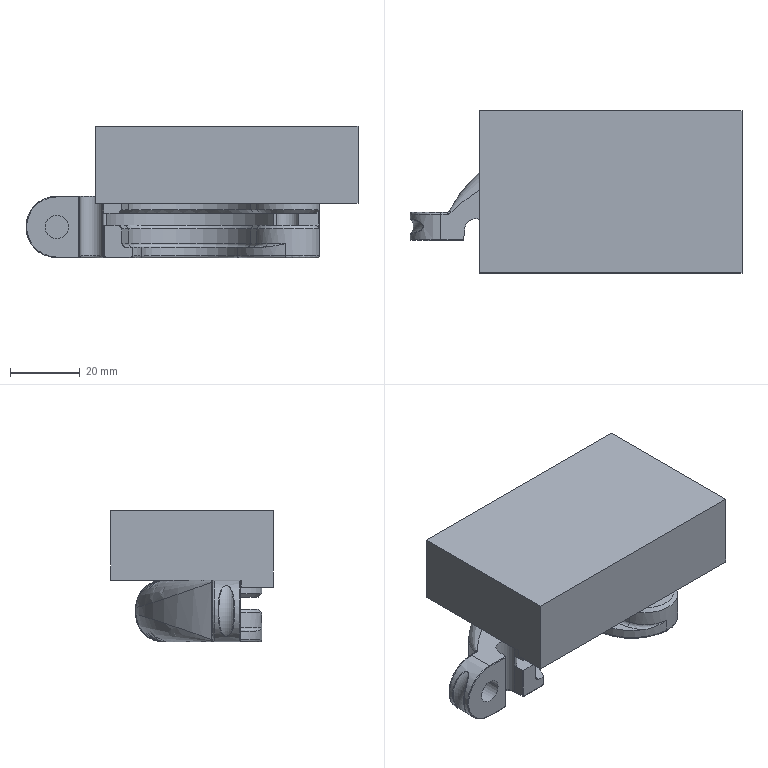NC program | NX | posted with a generic post | part box 94.951 x 46.35 x 37.6 mm
Lines 3770 to 5768 of 15115, first 1695 of 1981 lines:
(ZLEVEL_PROFILE , TOOL : 球刀3.)
N7424 T20 M6
N7426 G54
N7428 G17 G0 G90 X3.01 Y65.999 S6500 M3
N7430 G43 Z50. H20
N7432 Z-0.012
N7434 G94 G1 X3.002 Y65.816 F2500.
N7436 Y59.959
N7438 X2.816 Y59.741
N7440 X-0.303 Y59.468
N7442 G3 X-0.303 Y52.532 R3.481
N7444 G1 X2.817 Y52.259
N7446 X3.002 Y52.041
N7448 Y44.636
N7450 G2 X-2.874 Y41.989 R14.719
N7452 G3 X-2.874 Y14.011 R14.281
N7454 G2 X8.847 Y0.616 R14.719
N7456 X6.876 Y-5.533 R9.882
N7458 X-3.721 Y-7.993 R8.929
N7460 G1 X-3.779 Y-8.117 Z-0.024
N7462 X-3.661 Y-8.142
N7464 X-3.323 Y-8.273
N7466 G3 X5.193 Y-7.266 R9.125
N7468 X8.937 Y0.623 R9.314
N7470 X-2.856 Y14.099 R14.809
N7472 G2 X-2.856 Y41.901 R14.191
N7474 G3 X2.957 Y44.491 R14.809
N7476 G1 X3.085 Y44.759
N7478 Y52.041
N7480 X3.076 Y52.096
N7482 X2.824 Y52.349
N7484 X-0.296 Y52.622
N7486 G2 X-0.296 Y59.378 R3.391
N7488 G1 X2.823 Y59.651
N7490 G3 X3.085 Y59.959 R0.299
N7492 G1 Y66.
N7494 X3.148 Y65.963 Z-0.036
N7496 Y59.959
N7498 X3.119 Y59.863
N7500 X2.828 Y59.582
N7502 X-0.29 Y59.31
N7504 G3 X-0.29 Y52.69 R3.322
N7506 G1 X2.83 Y52.417
N7508 G2 X3.148 Y52.041 R0.41
N7510 G1 Y44.548
N7512 G2 X-2.842 Y41.833 R14.878
N7514 G3 X-2.842 Y14.167 R14.122
N7516 G2 X9.006 Y0.627 R14.878
N7518 X6.323 Y-6.418 R9.437
N7520 X-0.944 Y-8.962 R9.33
N7522 X-3.798 Y-8.159 R11.598
N7524 G1 X-3.818 Y-8.203 Z-0.048
N7526 G3 X-1.441 Y-8.962 R14.246
N7528 X1.397 Y-8.968 R14.76
N7530 X3.219 Y-8.431 R11.816
N7532 G1 X4.043 Y-8.114
N7534 X4.347 Y-7.917
N7536 X4.812 Y-7.69
N7538 X5.19 Y-7.397
N7540 X5.399 Y-7.266
N7542 X5.612 Y-7.088
N7544 X5.943 Y-6.842
N7546 X6.033 Y-6.776
N7548 X6.455 Y-6.382
N7550 X6.876 Y-5.908
N7552 X7.124 Y-5.57
N7554 X7.298 Y-5.358
N7556 X7.426 Y-5.146
N7558 X7.719 Y-4.766
N7560 G3 X8.562 Y-3.02 R32.361
N7562 G1 X8.648 Y-2.602
N7564 X8.754 Y-2.178
N7566 X8.871 Y-1.754
N7568 X8.984 Y-1.322
N7570 X9.064 Y0.631
N7572 G3 X-2.83 Y14.223 R14.936
N7574 G2 X-2.83 Y41.777 R14.064
N7576 G3 X3.201 Y44.515 R14.936
N7578 G1 Y52.041
N7580 G3 X2.834 Y52.475 R0.421
N7582 G1 X-0.285 Y52.748
N7584 G2 X-0.285 Y59.252 R3.264
N7586 G1 X2.832 Y59.525
N7588 G3 X3.201 Y59.959 R0.422
N7590 G1 Y66.
N7592 X3.248 Z-0.06
N7594 Y60.002
N7596 G2 X2.836 Y59.474 R0.495
N7598 G1 X-0.28 Y59.202
N7600 G3 X-0.28 Y52.798 R3.214
N7602 G1 X2.838 Y52.526
N7604 G2 X3.248 Y52.001 R0.492
N7606 G1 Y44.487
N7608 G2 X-2.82 Y41.727 R14.986
N7610 G3 X-2.82 Y14.273 R14.014
N7612 G2 X9.114 Y0.635 R14.986
N7614 G1 X9.018 Y-1.33
N7616 X8.984 Y-1.639
N7618 X8.598 Y-3.026
N7620 G2 X3.083 Y-8.577 R9.16
N7622 G3 X1.747 Y-8.962 R12.597
N7624 G2 X-1.553 Y-8.988 R13.63
N7626 X-3.838 Y-8.247 R13.052
N7628 G1 X-3.859 Y-8.291 Z-0.066
N7630 X-3.858 Y-8.289 Z-0.072
N7632 X-3.347 Y-8.538
N7634 G2 X-1.975 Y-8.965 R8.825
N7636 G3 X1.966 Y-8.962 R12.71
N7638 G1 X3.083 Y-8.614
N7640 X3.342 Y-8.538
N7642 X3.504 Y-8.451
N7644 X4.2 Y-8.116
N7646 G3 X6.543 Y-6.41 R8.105
N7648 G1 X6.876 Y-6.06
N7650 X7.298 Y-5.57
N7652 X7.554 Y-5.146
N7654 X7.719 Y-4.932
N7656 X7.831 Y-4.722
N7658 X8.141 Y-4.228
N7660 X8.274 Y-3.874
N7662 X8.474 Y-3.45
N7664 X8.562 Y-3.28
N7666 X9.004 Y-1.754
N7668 X9.053 Y-1.33
N7670 X9.16 Y0.638
N7672 G3 X-2.811 Y14.318 R15.032
N7674 G2 X-2.811 Y41.682 R13.968
N7676 G3 X3.069 Y44.297 R15.032
N7678 G1 X3.29 Y44.759
N7680 Y52.041
N7682 X2.842 Y52.571
N7684 X-0.276 Y52.844
N7686 G2 X-0.276 Y59.156 R3.168
N7688 G1 X2.839 Y59.429
N7690 G3 X3.29 Y59.959 R0.611
N7692 G1 Y66.
N7694 X3.328 Z-0.084
N7696 Y59.959
N7698 G2 X2.843 Y59.387 R0.652
N7700 G1 X-0.272 Y59.115
N7702 G3 X-0.272 Y52.885 R3.126
N7704 G1 X2.845 Y52.613
N7706 G2 X3.328 Y52.041 R0.554
N7708 G1 Y44.759
N7710 G2 X3.09 Y44.26 R0.611
N7712 X-2.803 Y41.642 R15.074
N7714 G3 X-2.803 Y14.358 R13.926
N7716 G2 X9.201 Y0.641 R15.074
N7718 G1 X9.089 Y-1.33
N7720 X9.035 Y-1.754
N7722 G2 X8.141 Y-4.325 R13.203
N7724 G1 X7.719 Y-5.014
N7726 G2 X4.769 Y-7.847 R8.785
N7728 X3.926 Y-8.292 R2.272
N7730 X-0.71 Y-9.138 R8.711
N7732 X-2.818 Y-8.724 R6.267
N7734 X-3.877 Y-8.329 R3.873
N7736 G1 X-3.9 Y-8.376 Z-0.091
N7738 X-3.899 Y-8.374 Z-0.098
N7740 X-3.579 Y-8.538
N7742 X-1.975 Y-9.031
N7744 G3 X2.24 Y-8.983 R11.251
N7746 X3.714 Y-8.461 R11.735
N7748 X8.071 Y-4.495 R9.056
N7750 X8.588 Y-3.45 R13.955
N7752 G1 X8.998 Y-2.178
N7754 G3 X9.246 Y0.644 R18.059
N7756 X-2.794 Y14.402 R15.118
N7758 G2 X-2.794 Y41.598 R13.882
N7760 G3 X3.369 Y44.414 R15.118
N7762 G1 Y52.041
N7764 G3 X2.849 Y52.657 R0.645
N7766 G1 X-0.269 Y52.93
N7768 G2 X-0.269 Y59.07 R3.082
N7770 G1 X2.846 Y59.343
N7772 G3 X3.369 Y59.959 R0.598
N7774 G1 Y66.
N7776 X3.41 Z-0.113
N7778 Y59.959
N7780 G2 X2.849 Y59.298 R0.642
N7782 G1 X-0.265 Y59.025
N7784 G3 X-0.265 Y52.975 R3.037
N7786 G1 X2.852 Y52.702
N7788 G2 X3.41 Y52.041 R0.708
N7790 G1 Y44.759
N7792 G2 X3.136 Y44.182 R0.959
N7794 X-2.784 Y41.554 R15.163
N7796 G3 X-2.784 Y14.446 R13.837
N7798 G2 X9.291 Y0.647 R15.163
N7800 X9.112 Y-1.754 R17.857
N7802 X1.819 Y-9.097 R9.23
N7804 X-3.921 Y-8.42 R9.397
N7806 G1 X-3.941 Y-8.463 Z-0.122
N7808 X-3.943 Y-8.469 Z-0.13
N7810 G3 X5.308 Y-7.69 R9.483
N7812 X9.338 Y0.65 R9.532
N7814 X-2.775 Y14.492 R15.21
N7816 G2 X-2.775 Y41.508 R13.79
N7818 G3 X3.159 Y44.141 R15.21
N7820 G1 X3.453 Y44.759
N7822 Y52.041
N7824 G3 X2.856 Y52.749 R0.775
N7826 G1 X-0.261 Y53.022
N7828 G2 X-0.261 Y58.978 R2.99
N7830 G1 X2.853 Y59.251
N7832 G3 X3.453 Y59.959 R0.687
N7834 G1 Y65.955
N7836 X3.495 Y66. Z-0.149
N7838 Y59.959
N7840 G2 X2.856 Y59.205 R0.732
N7842 G1 X-0.257 Y58.932
N7844 G3 X-0.257 Y53.068 R2.944
N7846 G1 X2.859 Y52.795
N7848 G2 X3.495 Y52.041 R0.816
N7850 G1 Y44.759
N7852 G2 X3.183 Y44.101 R0.987
N7854 X-2.766 Y41.462 R15.256
N7856 G3 X-2.766 Y14.538 R13.744
N7858 G2 X9.384 Y0.654 R15.256
N7860 X-2.803 Y-8.962 R9.428
N7862 G1 X-3.968 Y-8.522
N7864 X-3.987 Y-8.563 Z-0.169
N7866 G3 X0.976 Y-9.383 R9.836
N7868 X9.431 Y0.657 R9.502
N7870 X-2.756 Y14.585 R15.304
N7872 G2 X-2.756 Y41.415 R13.696
N7874 G3 X3.207 Y44.059 R15.304
N7876 X3.539 Y44.759 R0.856
N7878 G1 Y52.041
N7880 G3 X2.863 Y52.843 R0.847
N7882 G1 X-0.252 Y53.115
N7884 G2 X-0.252 Y58.885 R2.896
N7886 G1 X2.86 Y59.157
N7888 G3 X3.539 Y59.959 R0.831
N7890 G1 Y66.
N7892 X3.581 Z-0.19
N7894 Y59.959
N7896 G2 X2.863 Y59.11 R0.88
N7898 G1 X-0.248 Y58.838
N7900 G3 X-0.248 Y53.162 R2.849
N7902 G1 X2.867 Y52.89
N7904 G2 X3.581 Y52.041 R0.877
N7906 G1 Y44.759
N7908 G2 X3.23 Y44.019 R0.905
N7910 X-2.747 Y41.37 R15.351
N7912 G3 X-2.747 Y14.63 R13.649
N7914 G2 X9.478 Y0.66 R15.351
N7916 X8.562 Y-4.083 R10.171
N7918 X-4.005 Y-8.603 R9.526
N7920 G1 X-4.024 Y-8.645 Z-0.212
N7922 G3 X3.504 Y-8.857 R9.683
N7924 X9.438 Y-1.33 R9.544
N7926 X9.524 Y0.663 R25.818
N7928 X-2.737 Y14.675 R15.397
N7930 G2 X-2.737 Y41.325 R13.603
N7932 G3 X3.253 Y43.979 R15.397
N7934 X3.623 Y44.759 R1.202
N7936 G1 Y52.041
N7938 G3 X2.87 Y52.935 R0.865
N7940 G1 X-0.244 Y53.208
N7942 G2 X-0.244 Y58.792 R2.803
N7944 G1 X2.867 Y59.064
N7946 G3 X3.623 Y59.959 R0.931
N7948 G1 Y66.
N7950 X3.664 Z-0.236
N7952 Y59.959
N7954 G2 X2.87 Y59.019 R0.98
N7956 G1 X-0.24 Y58.747
N7958 G3 X-0.24 Y53.253 R2.758
N7960 G1 X2.874 Y52.98
N7962 G2 X3.664 Y52.041 R0.959
N7964 G1 Y44.759
N7966 G2 X3.276 Y43.939 R1.321
N7968 X-2.728 Y41.28 R15.442
N7970 G3 X-2.728 Y14.72 R13.558
N7972 G2 X9.569 Y0.667 R15.442
N7974 X9.422 Y-1.754 R26.252
N7976 X3.504 Y-8.916 R9.735
N7978 X-4.044 Y-8.686 R9.795
N7980 G1 X-4.062 Y-8.725 Z-0.261
N7982 G3 X4.347 Y-8.585 R9.808
N7984 X9.458 Y-1.754 R9.666
N7986 X9.614 Y0.67 R26.736
N7988 X-2.719 Y14.764 R15.487
N7990 G2 X-2.719 Y41.236 R13.513
N7992 G3 X3.298 Y43.9 R15.487
N7994 X3.704 Y44.759 R1.392
N7996 G1 Y52.041
N7998 G3 X2.877 Y53.025 R1.009
N8000 G1 X-0.236 Y53.297
N8002 G2 X-0.236 Y58.703 R2.713
N8004 G1 X2.874 Y58.975
N8006 G3 X3.562 Y59.484 R0.818
N8008 X3.704 Y59.959 R2.687
N8010 G1 Y66.
N8012 X3.718 Z-0.273
N8014 X3.744 Z-0.286
N8016 Y59.959
N8018 G2 X3.578 Y59.431 R2.685
N8020 X2.886 Y58.932 R0.833
N8022 G1 X-0.233 Y58.659
N8024 G3 X-0.233 Y53.341 R2.669
N8026 G1 X2.881 Y53.069
N8028 G2 X3.601 Y52.52 R0.891
N8030 G1 X3.744 Y52.041
N8032 Y44.759
N8034 G2 X3.32 Y43.862 R1.476
N8036 X-2.71 Y41.193 R15.531
N8038 G3 X-2.71 Y14.807 R13.469
N8040 G2 X9.658 Y0.673 R15.531
N8042 X9.496 Y-1.754 R22.683
N8044 X3.504 Y-9.01 R9.656
N8046 X-4.08 Y-8.762 R9.877
N8048 G1 X-4.097 Y-8.799 Z-0.313
N8050 G3 X-0.71 Y-9.661 R9.462
N8052 X9.598 Y-1.33 R9.633
N8054 X9.701 Y0.676 R19.124
N8056 X-2.702 Y14.849 R15.574
N8058 G2 X-2.702 Y41.151 R13.426
N8060 G3 X3.342 Y43.824 R15.574
N8062 X3.71 Y44.34 R1.528
N8064 G2 X3.783 Y44.759 R0.762
N8066 G1 Y52.041
N8068 G3 X3.64 Y52.52 R0.703
N8070 X2.884 Y53.112 R0.928
N8072 G1 X-0.229 Y53.384
N8074 G2 X-0.229 Y58.616 R2.626
N8076 G1 X2.88 Y58.888
N8078 G3 X3.569 Y59.304 R1.042
N8080 G1 X3.783 Y59.959
N8082 Y66.
N8084 X3.796 Z-0.327
N8086 X3.821 Z-0.341
N8088 Y59.959
N8090 X3.669 Y59.47
N8092 G2 X2.896 Y58.847 R0.891
N8094 G1 X-0.225 Y58.574
N8096 G3 X-0.225 Y53.426 R2.584
N8098 G1 X2.889 Y53.154
N8100 G2 X3.625 Y52.669 R0.925
N8102 X3.821 Y52.041 R1.757
N8104 G1 Y44.759
N8106 X3.777 Y44.513
N8108 G2 X3.363 Y43.787 R1.255
N8110 X-2.693 Y41.11 R15.616
N8112 G3 X-2.693 Y14.89 R13.384
N8114 G2 X9.743 Y0.679 R15.616
N8116 X9.496 Y-2.178 R12.745
N8118 X-4.115 Y-8.837 R9.746
N8120 G1 X-4.133 Y-8.876 Z-0.369
N8122 G3 X7.719 Y-6.036 R9.835
N8124 X9.784 Y0.682 R10.13
N8126 X-2.685 Y14.931 R15.658
N8128 G2 X-2.685 Y41.069 R13.342
N8130 G3 X3.384 Y43.751 R15.658
N8132 X3.858 Y44.759 R1.53
N8134 G1 Y52.041
N8136 G3 X3.724 Y52.52 R0.937
N8138 X2.891 Y53.195 R0.966
N8140 G1 X-0.222 Y53.468
N8142 G2 X-0.222 Y58.532 R2.542
N8144 G1 X2.893 Y58.805
N8146 G3 X3.719 Y59.483 R0.947
N8148 G1 X3.858 Y59.959
N8150 Y66.
N8152 X3.87 Z-0.384
N8154 X3.895 Z-0.399
N8156 Y59.959
N8158 X3.718 Y59.304
N8160 G2 X2.889 Y58.763 R1.217
N8162 G1 X-0.218 Y58.491
N8164 G3 X-0.218 Y53.509 R2.501
N8166 G1 X2.894 Y53.236
N8168 G2 X3.768 Y52.52 R1.007
N8170 X3.895 Y52.041 R0.915
N8172 G1 Y44.759
N8174 G2 X3.404 Y43.715 R1.553
N8176 X-2.677 Y41.029 R15.699
N8178 G3 X-2.677 Y14.971 R13.301
N8180 G2 X9.825 Y0.684 R15.699
N8182 X-2.947 Y-9.386 R9.875
N8184 G1 X-4.082 Y-8.952
N8186 X-4.151 Y-8.916
N8188 X-4.171 Y-8.959 Z-0.43
N8190 G3 X0.133 Y-9.878 R10.428
N8192 X9.865 Y0.687 R9.927
N8194 X-2.669 Y15.01 R15.739
N8196 G2 X-2.669 Y40.99 R13.261
N8198 G3 X3.424 Y43.68 R15.739
N8200 X3.93 Y44.759 R1.549
N8202 G1 Y52.041
N8204 G3 X2.897 Y53.276 R1.256
N8206 G1 X-0.214 Y53.548
N8208 G2 X-0.214 Y58.452 R2.461
N8210 G1 X2.892 Y58.723
N8212 G3 X3.356 Y58.887 R1.345
N8214 X3.93 Y59.959 R1.353
N8216 G1 Y66.
N8218 X3.941 Z-0.446
N8220 X3.965 Z-0.462
N8222 Y59.959
N8224 G2 X2.895 Y58.684 R1.27
N8226 G1 X-0.211 Y58.412
N8228 G3 X-0.211 Y53.588 R2.422
N8230 G1 X2.9 Y53.315
N8232 G2 X3.965 Y52.041 R1.276
N8234 G1 Y44.759
N8236 G2 X3.444 Y43.646 R1.529
N8238 X-2.661 Y40.951 R15.778
N8240 G3 X-2.661 Y15.049 R13.222
N8242 G2 X9.904 Y0.69 R15.778
N8244 X-1.483 Y-9.81 R9.965
N8246 X-4.187 Y-8.994 R11.457
N8248 G1 X-4.203 Y-9.028 Z-0.495
N8250 G3 X6.316 Y-7.69 R9.986
N8252 X9.943 Y0.693 R10.055
N8254 X-2.653 Y15.086 R15.817
N8256 G2 X-2.653 Y40.914 R13.183
N8258 G3 X3.463 Y43.612 R15.817
N8260 X3.999 Y44.759 R1.531
N8262 G1 Y52.041
N8264 G3 X2.903 Y53.354 R1.31
N8266 G1 X-0.208 Y53.626
N8268 G2 X-0.208 Y58.374 R2.383
N8270 G1 X2.898 Y58.646
N8272 G3 X3.999 Y59.959 R1.293
N8274 G1 Y66.
N8276 X4.009 Z-0.512
N8278 X4.032 Z-0.528
N8280 Y59.959
N8282 G2 X2.9 Y58.608 R1.304
N8284 G1 X-0.204 Y58.337
N8286 G3 X-0.204 Y53.663 R2.346
N8288 G1 X2.906 Y53.391
N8290 G2 X4.032 Y52.041 R1.346
N8292 G1 Y44.759
N8294 G2 X3.482 Y43.579 R1.574
N8296 X-2.645 Y40.877 R15.854
N8298 G3 X-2.645 Y15.123 R13.146
N8300 G2 X9.98 Y0.695 R15.854
N8302 X6.382 Y-7.69 R10.101
N8304 X-4.219 Y-9.063 R10.037
N8306 G1 X-4.23 Y-9.086 Z-0.546
N8308 X-4.236 Y-9.098 Z-0.563
N8310 G3 X4.499 Y-8.962 R10.088
N8312 X10.017 Y0.698 R10.088
N8314 X-2.638 Y15.159 R15.891
N8316 G2 X-2.638 Y40.841 R13.109
N8318 G3 X3.5 Y43.547 R15.891
N8320 X4.064 Y44.759 R1.472
N8322 G1 Y52.041
N8324 G3 X2.908 Y53.428 R1.38
N8326 G1 X-0.201 Y53.7
N8328 G2 X-0.201 Y58.3 R2.309
N8330 G1 X2.903 Y58.572
N8332 G3 X4.064 Y59.959 R1.339
N8334 G1 Y66.
N8336 X4.072 Z-0.581
N8338 X4.095 Z-0.599
N8340 Y59.959
N8342 G2 X2.906 Y58.536 R1.373
N8344 G1 X-0.198 Y58.264
N8346 G3 X-0.198 Y53.736 R2.273
N8348 G1 X2.911 Y53.464
N8350 G2 X4.095 Y52.041 R1.406
N8352 G1 Y44.759
N8354 G2 X3.518 Y43.516 R1.509
N8356 X-2.631 Y40.806 R15.927
N8358 G3 X-2.631 Y15.194 R13.073
N8360 G2 X10.053 Y0.7 R15.927
N8362 X-4.25 Y-9.127 R10.085
N8364 G1 X-4.26 Y-9.151 Z-0.617
N8366 X-4.263 Y-9.156 Z-0.635
N8368 G3 X2.416 Y-9.81 R10.112
N8370 X10.087 Y0.703 R10.157
N8372 X-2.624 Y15.229 R15.962
N8374 G2 X-2.624 Y40.771 R13.038
N8376 G3 X3.535 Y43.485 R15.962
N8378 X4.125 Y44.759 R1.545
N8380 G1 Y52.041
N8382 G3 X2.914 Y53.498 R1.435
N8384 G1 X-0.195 Y53.77
N8386 G2 X-0.195 Y58.23 R2.238
N8388 G1 X2.908 Y58.501
N8390 G3 X4.125 Y59.959 R1.431
N8392 G1 Y66.
N8394 X4.154 Z-0.672
N8396 Y59.959
N8398 G2 X2.911 Y58.467 R1.461
N8400 G1 X-0.192 Y58.196
N8402 G3 X-0.192 Y53.804 R2.204
N8404 G1 X2.916 Y53.532
N8406 G2 X4.154 Y52.041 R1.459
N8408 G1 Y44.759
N8410 G2 X3.551 Y43.455 R1.58
N8412 X-2.617 Y40.738 R15.996
N8414 G3 X-2.617 Y15.262 R13.004
N8416 G2 X10.121 Y0.705 R15.996
N8418 X9.36 Y-3.874 R10.597
N8420 X-4.277 Y-9.186 R10.127
N8422 G1 X-4.286 Y-9.205 Z-0.691
N8424 X-4.291 Y-9.216 Z-0.71
N8426 G3 X9.562 Y-3.45 R10.175
N8428 X10.154 Y0.707 R10.9
N8430 X-2.61 Y15.294 R16.029
N8432 G2 X-2.61 Y40.706 R12.971
N8434 G3 X3.567 Y43.426 R16.029
N8436 X4.182 Y44.759 R1.615
N8438 G1 Y52.041
N8440 G3 X2.919 Y53.565 R1.48
N8442 G1 X-0.189 Y53.837
N8444 G2 X-0.189 Y58.163 R2.171
N8446 G1 X2.913 Y58.434
N8448 G3 X4.182 Y59.959 R1.493
N8450 G1 Y66.
N8452 X4.209 Z-0.749
N8454 Y59.959
N8456 G2 X2.916 Y58.403 R1.519
N8458 G1 X-0.186 Y58.131
N8460 G3 X-0.186 Y53.869 R2.139
N8462 G1 X2.921 Y53.597
N8464 G2 X4.209 Y52.041 R1.495
N8466 G1 Y44.759
N8468 G2 X3.583 Y43.398 R1.757
N8470 X-2.604 Y40.675 R16.061
N8472 G3 X-2.604 Y15.325 R12.939
N8474 G2 X10.186 Y0.71 R16.061
N8476 X9.436 Y-3.874 R10.816
N8478 X-1.553 Y-10.082 R10.242
N8480 X-4.305 Y-9.248 R9.983
N8482 G1 X-4.315 Y-9.268 Z-0.769
N8484 X-4.319 Y-9.277 Z-0.789
N8486 G3 X7.719 Y-6.704 R10.224
N8488 X10.217 Y0.712 R10.376
N8490 X-2.598 Y15.356 R16.092
N8492 G2 X-2.598 Y40.644 R12.908
N8494 G3 X3.598 Y43.371 R16.092
N8496 X4.235 Y44.759 R1.775
N8498 G1 Y52.041
N8500 G3 X2.923 Y53.628 R1.552
N8502 G1 X-0.184 Y53.9
N8504 G2 X-0.184 Y58.1 R2.108
N8506 G1 X2.919 Y58.372
N8508 G3 X3.671 Y58.693 R1.312
N8510 X4.235 Y59.959 R1.662
N8512 G1 Y66.
N8514 X4.26 Z-0.829
N8516 Y59.959
N8518 G2 X3.992 Y59.014 R1.92
N8520 X2.925 Y58.342 R1.38
N8522 G1 X-0.181 Y58.071
N8524 G3 X-0.181 Y53.929 R2.078
N8526 G1 X2.926 Y53.658
N8528 G2 X4.26 Y52.041 R1.592
N8530 G1 Y44.759
N8532 G2 X3.613 Y43.344 R1.794
N8534 X-2.592 Y40.615 R16.122
N8536 G3 X-2.592 Y15.385 R12.878
N8538 G2 X10.247 Y0.714 R16.122
N8540 X-4.332 Y-9.303 R10.277
N8542 G1 X-4.34 Y-9.322 Z-0.85
N8544 X-4.345 Y-9.33 Z-0.87
N8546 G3 X9.146 Y-4.722 R10.304
N8548 X10.276 Y0.716 R10.687
N8550 X-2.586 Y15.413 R16.15
N8552 G2 X-2.586 Y40.587 R12.85
N8554 G3 X3.627 Y43.319 R16.15
N8556 X4.284 Y44.759 R1.825
N8558 G1 Y52.041
N8560 X4.269 Y52.096
N8562 X4.208 Y52.52
N8564 G3 X2.928 Y53.687 R1.505
N8566 G1 X-0.179 Y53.958
N8568 G2 X-0.179 Y58.042 R2.05
N8570 G1 X2.928 Y58.313
N8572 G3 X4.017 Y59.01 R1.395
N8574 X4.284 Y59.959 R2.025
N8576 G1 Y66.
N8578 X4.306 Z-0.912
N8580 Y59.959
N8582 G2 X4.011 Y58.96 R2.045
N8584 X2.927 Y58.285 R1.412
N8586 G1 X-0.176 Y58.014
N8588 G3 X-0.176 Y53.986 R2.022
N8590 G1 X2.93 Y53.714
N8592 G2 X4.231 Y52.52 R1.516
N8594 G1 X4.294 Y52.096
N8596 X4.306 Y52.041
N8598 Y44.759
N8600 G2 X3.64 Y43.294 R1.876
N8602 X-2.58 Y40.559 R16.178
N8604 G3 X-2.58 Y15.441 R12.822
N8606 G2 X10.303 Y0.718 R16.178
N8608 X10.248 Y-1.253 R16.497
N8610 X-4.358 Y-9.358 R10.334
N8612 G1 X-4.37 Y-9.387 Z-0.955
N8614 G3 X10.019 Y-2.602 R10.381
N8616 X10.33 Y0.72 R11.986
N8618 X-2.575 Y15.467 R16.205
N8620 G2 X-2.575 Y40.533 R12.795
N8622 G3 X3.653 Y43.271 R16.205
N8624 X4.328 Y44.759 R1.921
N8626 G1 Y52.041
N8628 X4.255 Y52.52
N8630 G3 X2.932 Y53.741 R1.532
N8632 G1 X-0.174 Y54.013
N8634 G2 X-0.174 Y57.987 R1.995
N8636 G1 X2.931 Y58.259
N8638 G3 X4.007 Y58.912 R1.422
N8640 X4.328 Y59.959 R2.057
N8642 G1 Y66.
N8644 X4.349 Z-1.
N8646 Y59.959
N8648 G2 X4.011 Y58.875 R2.056
N8650 X2.934 Y58.232 R1.44
N8652 G1 X-0.172 Y57.96
N8654 G3 X-0.172 Y54.04 R1.968
N8656 G1 X2.934 Y53.768
N8658 G2 X4.137 Y52.944 R1.583
N8660 X4.349 Y52.041 R2.564
N8662 G1 Y44.759
N8664 G2 X3.666 Y43.247 R1.947
N8666 X-2.569 Y40.507 R16.232
N8668 G3 X-2.569 Y15.493 R12.768
N8670 G2 X10.357 Y0.722 R16.232
N8672 X9.626 Y-3.874 R10.865
N8674 X-4.364 Y-9.415 R10.391
N8676 G3 X-4.808 Y-9.27 R2.
N8678 G0 Z50.
N8680 M5
(PLANAR_PROFILE , TOOL : D4.)
N8682 T06 M6
N8684 G54
N8686 G17 G0 G90 X-0.12 Y-1.144 S4500 M3
N8688 G43 Z50. H6
N8690 Z-0.4
N8692 G94 G1 Y-4.03 F500.
N8694 X-0.13 Y-4.105
N8696 X-0.075 Y-4.16
N8698 X0. Y-4.15
N8700 G3 X4.15 Y0. R4.15
N8702 X0. Y-4.15 R-4.15
N8704 G1 X0.075 Y-4.16
N8706 X0.13 Y-4.105
N8708 X0.12 Y-4.03
N8710 Y-1.144
N8712 G0 X-0.12 Z-0.8
N8714 G1 Y-4.03
N8716 X-0.13 Y-4.105
N8718 X-0.075 Y-4.16
N8720 X0. Y-4.15
N8722 G3 X4.15 Y0. R4.15
N8724 X0. Y-4.15 R-4.15
N8726 G1 X0.075 Y-4.16
N8728 X0.13 Y-4.105
N8730 X0.12 Y-4.03
N8732 Y-1.144
N8734 G0 Z50.
N8736 M5
(PLANAR_PROFILE_COPY_COPY , TOOL : D5.)
N8738 T07 M6
N8740 G54
N8742 G17 G0 G90 X-0.371 Y-0.149 S5500 M3
N8744 G43 Z50. H7
N8746 Z-3.8
N8748 G41 G94 G1 X-1. Y-0.4 F300. D7
N8750 G3 X0. Y-1.4 R1.
N8752 X1.4 Y0. R1.4
N8754 X0. Y-1.4 R-1.4
N8756 X1. Y-0.4 R1.
N8758 G40
N8760 G1 X0.371 Y-0.149
N8762 G0 Z50.
N8764 M5
(PLANAR_PROFILE_COPY , TOOL : D5.)
N8766 T15 M6
N8768 G54
N8770 G17 G0 G90 X-0.709 Y-0.173 S5500 M3
N8772 G43 Z50. H15
N8774 Z-0.8
N8776 G41 G94 G1 X-3. Y-0.73 F300. D15
N8778 G3 X0. Y-3.73 R3.
N8780 X3.73 Y0. R3.73
N8782 X0. Y-3.73 R-3.73
N8784 X3. Y-0.73 R3.
N8786 G40
N8788 G1 X0.709 Y-0.173
N8790 G0 Z50.
(PLANAR_PROFILE_COPY_COPY_COPY , TOOL : D5.)
N8792 X-0.447 Y-0.224
N8794 Z-3.8
N8796 G41 G1 X-1. Y-0.5
N8798 G3 X0. Y-1.5 R1.
N8800 X1.5 Y0. R1.5
N8802 X0. Y-1.5 R-1.5
N8804 X1. Y-0.5 R1.
N8806 G40
N8808 G1 X0.447 Y-0.224
N8810 G0 Z50.
N8812 M5
(PLANAR_MILL_4 , TOOL : 倒角3.)
N8814 T12 M6
N8816 G54
N8818 G17 G0 G90 X-0.5 Y-5.226 S3500 M3
N8820 G43 Z50. H12
N8822 Z1.5
N8824 G94 G1 Z-0.5 F800.
N8826 Y-5.25
N8828 G3 X0. Y-5.75 R0.5
N8830 X5.75 Y0. R5.75
N8832 X0. Y-5.75 R-5.75
N8834 X0.5 Y-5.226 R0.501
N8836 G1 Z1.5
N8838 G0 Z50.
(PLANAR_MILL_4_COPY , TOOL : 倒角3.)
N8840 X-0.5 Y-2.958
N8842 Z0.7
N8844 G1 Z-1.3
N8846 Y-3.
N8848 G3 X0. Y-3.5 R0.5
N8850 X3.5 Y0. R3.5
N8852 X0. Y-3.5 R-3.5
N8854 X0.5 Y-2.958 R0.502
N8856 G1 Z0.7
N8858 G0 Z50.
N8860 M5
(CAVITY_MILL_2 , TOOL : D8开粗)
N8862 T19 M6
N8864 G54
N8866 G17 G0 G90 X3. Y-7. S5500 M3
N8868 G43 Z10.2 H19
N8870 Z-0.5
N8872 G94 G1 Y-4.6 F2500.
N8874 G3 X0. Y-1.6 R3.
N8876 G1 X-4.
N8878 G2 X-5.6 Y0. R1.6
N8880 G1 Y1.367
N8882 G2 X-7.934 Y3.771 R5.046
N8884 G1 X-8. Y3.918
N8886 Y5.49
N8888 G3 X-7.498 Y3.972 R7.089
N8890 X-3.5 Y1.321 R4.566
N8892 G1 X-2.184
N8894 G3 X-0.001 Y1.949 R4.636
N8896 X2.184 Y1.321 R4.451
N8898 G1 X3.805
N8900 G3 X7.551 Y3.669 R4.163
N8902 X8. Y4.898 R6.489
N8904 G1 Y3.495
N8906 X7.983 Y3.459
N8908 G2 X5.6 Y1.202 R4.643
N8910 G1 Y0.
N8912 G2 X4. Y-1.6 R1.6
N8914 G1 X0.
N8916 G3 X-3. Y-4.6 R3.
N8918 G1 Y-7.
N8920 G0 X3. Z-0.999
N8922 G1 Y-4.6
N8924 G3 X0. Y-1.6 R3.
N8926 G1 X-4.
N8928 G2 X-5.6 Y0. R1.6
N8930 G1 Y0.339
N8932 G2 X-7.93 Y2.626 R5.107
N8934 G1 X-8. Y2.772
N8936 Y4.202
N8938 G3 X-7.5 Y2.839 R6.766
N8940 X-3.5 Y0.311 R4.627
N8942 G1 X-2.031
N8944 G3 X0. Y0.847 R4.237
N8946 X2.031 Y0.311 R4.404
N8948 G1 X3.8
N8950 G3 X7.886 Y3.305 R4.461
N8952 X8. Y3.697 R6.387
N8954 G1 Y2.386
N8956 G2 X5.6 Y0.221 R4.941
N8958 G1 Y0.
N8960 G2 X4. Y-1.6 R1.6
N8962 G1 X0.
N8964 G3 X-3. Y-4.6 R3.
N8966 G1 Y-7.
N8968 G0 X3. Z-1.499
N8970 G1 Y-4.6
N8972 G3 X0. Y-1.6 R3.
N8974 G1 X-4.
N8976 G2 X-5.53 Y-0.467 R1.6
N8978 X-7.926 Y1.761 R5.23
N8980 G1 X-8. Y1.908
N8982 Y3.292
N8984 G3 X-7.5 Y1.981 R6.293
N8986 X-3.5 Y-0.463 R4.75
N8988 G1 X-1.858
N8990 G3 X-0.007 Y-0.038 R4.501
N8992 X1.858 Y-0.463 R5.021
N8994 G1 X3.8
N8996 G3 X6.521 Y0.538 R4.647
N8998 X8. Y2.831 R4.859
N9000 G1 Y1.603
N9002 G2 X6.819 Y0.161 R5.339
N9004 X5.482 Y-0.602 R5.127
N9006 X4. Y-1.6 R1.6
N9008 G1 X0.
N9010 G3 X-3. Y-4.6 R3.
N9012 G1 Y-7.
N9014 G0 X3. Z-1.999
N9016 G1 Y-4.6
N9018 G3 X0. Y-1.6 R3.
N9020 G1 X-4.
N9022 G2 X-4.816 Y-1.376 R1.6
N9024 X-7.864 Y0.987 R5.182
N9026 X-8. Y1.239 R6.193
N9028 G1 Y2.562
N9030 G3 X-7.447 Y1.225 R5.713
N9032 X-3.5 Y-1.094 R4.702
N9034 G1 X-1.62
N9036 G3 X-0.001 Y-0.755 R4.572
N9038 X1.654 Y-1.094 R4.522
N9040 G1 X3.8
N9042 G3 X6.459 Y-0.15 R4.553
N9044 X8. Y2.158 R4.739
N9046 G1 Y0.944
N9048 G2 X6.752 Y-0.531 R5.219
N9050 X4.561 Y-1.498 R5.033
N9052 X4. Y-1.6 R1.6
N9054 G1 X0.
N9056 G3 X-3. Y-4.6 R3.
N9058 G1 Y-7.
N9060 G0 X1.429 Z-2.499
N9062 G1 X2.01 Y-5.177
N9064 G3 X0.061 Y-1.408 R3.
N9066 X1.405 Y-1.626 R4.634
N9068 G1 X3.8
N9070 G3 X8. Y1.557 R4.514
N9072 G1 Y0.37
N9074 G2 X3.8 Y-2.106 R4.994
N9076 G1 X1.399
N9078 G2 X-0.004 Y-1.89 R5.114
N9080 X-1.404 Y-2.106 R4.707
N9082 G1 X-3.508
N9084 G2 X-7.918 Y0.522 R5.162
N9086 G1 X-8. Y0.673
N9088 Y1.971
N9090 G3 X-7.5 Y0.757 R5.491
N9092 X-3.5 Y-1.626 R4.682
N9094 G1 X-1.372
N9096 G3 X-0.008 Y-1.385 R4.227
N9098 G1 X0.061 Y-1.408
N9100 G0 Z10.2
N9102 X11.2 Y3.188
N9104 Z-2.998
N9106 G3 X8. Y1.091 R3.
N9108 G2 X3.8 Y-2.08 R4.5
N9110 G1 X1.082
N9112 G2 X0.022 Y-1.939 R4.094
N9114 X-1.082 Y-2.08 R4.848
N9116 G1 X-3.5
N9118 G2 X-7.926 Y1.225 R4.787
N9120 X-8. Y1.463 R5.254
N9122 G3 X-11.2 Y3.626 R3.
N9124 G0 Z10.2
N9126 X11.2 Y2.787
N9128 Z-3.498
N9130 G3 X8. Y0.691 R3.
N9132 G2 X3.8 Y-2.472 R4.49
N9134 G1 X0.569
N9136 X0.022 Y-2.442
N9138 G2 X-0.569 Y-2.472 R6.704
N9140 G1 X-3.5
N9142 G2 X-8. Y0.982 R4.833
N9144 G3 X-11.2 Y3.11 R3.
N9146 G0 Z10.2
N9148 X11.2 Y2.439
N9150 Z-3.998
N9152 G3 X8. Y0.344 R3.
N9154 G2 X3.8 Y-2.812 R4.48
N9156 G1 X-3.5
N9158 G2 X-8. Y0.66 R4.755
N9160 G3 X-11.2 Y2.834 R3.
N9162 G0 Z10.2
N9164 X11.2 Y2.129
N9166 Z-4.497
N9168 G3 X8. Y0.036 R3.
N9170 G2 X3.8 Y-3.105 R4.462
N9172 G1 X-3.5
N9174 G2 X-8. Y0.316 R4.792
N9176 G3 X-11.2 Y2.441 R3.
N9178 G0 Z10.2
N9180 X11.2 Y1.837
N9182 Z-4.997
N9184 G3 X7.993 Y-0.239 R3.
N9186 G2 X3.8 Y-3.357 R4.462
N9188 G1 X-3.5
N9190 G2 X-8. Y0.054 R4.78
N9192 G3 X-11.2 Y2.178 R3.
N9194 G0 Z10.2
N9196 X11.2 Y1.472
N9198 Z-5.497
N9200 G3 X7.964 Y-0.538 R3.
N9202 G2 X3.8 Y-3.572 R4.469
N9204 G1 X-3.5
N9206 G2 X-7.996 Y-0.181 R4.773
N9208 G3 X-11.2 Y1.933 R3.
N9210 G0 Z10.2
N9212 X11.2 Y0.919
N9214 Z-5.996
N9216 G3 X7.889 Y-0.934 R3.
N9218 G2 X3.8 Y-3.752 R4.452
N9220 G1 X-3.5
N9222 G2 X-7.976 Y-0.435 R4.76
N9224 G3 X-11.2 Y1.634 R3.
N9226 G0 Z10.2
N9228 X11.187 Y0.107
N9230 Z-6.496
N9232 G3 X7.729 Y-1.447 R3.
N9234 G2 X5.384 Y-3.589 R4.44
N9236 X3.8 Y-3.9 R4.968
N9238 G1 X-3.5
N9240 G2 X-6.816 Y-2.513 R4.913
N9242 X-7.939 Y-0.697 R4.824
N9244 G3 X-11.2 Y1.3 R3.
N9246 G0 Z10.2
N9248 X10.998 Y-1.3
N9250 Z-6.996
N9252 G3 X7.322 Y-2.228 R3.
N9254 G2 X4.213 Y-3.994 R4.44
N9256 G3 X1.519 Y-7.017 R3.
N9258 G0 Z10.2
N9260 X-1.122
N9262 Z-6.996
N9264 G3 X-3.865 Y-4. R3.
N9266 G2 X-7.868 Y-1.017 R4.742
N9268 G3 X-11.2 Y0.831 R3.
N9270 G0 X-2.467 Y-7.105 Z-7.496
N9272 G3 X-4.677 Y-3.942 R3.
N9274 G2 X-7.789 Y-1.283 R4.758
N9276 G3 X-11.197 Y0.422 R3.
N9278 G0 X-3.593 Y-7.163 Z-7.995
N9280 G3 X-5.337 Y-3.77 R3.
N9282 G2 X-6.816 Y-2.774 R4.832
N9284 X-7.65 Y-1.637 R4.783
N9286 G3 X-11.164 Y-0.16 R3.
N9288 G0 X-4.752 Y-7.088 Z-8.495
N9290 G3 X-5.972 Y-3.48 R3.
N9292 G2 X-7.461 Y-2.006 R4.728
N9294 G3 X-11.081 Y-0.821 R3.
N9296 G0 X-5.498 Y-6.936 Z-8.995
N9298 G3 X-6.361 Y-3.229 R3.
N9300 G2 X-7.229 Y-2.361 R4.7
N9302 G3 X-10.936 Y-1.498 R3.
N9304 G0 X-5.498 Y-6.936 Z-9.494
N9306 G3 X-6.361 Y-3.229 R3.
N9308 G2 X-7.229 Y-2.361 R4.7
N9310 G3 X-10.936 Y-1.498 R3.
N9312 G0 X-5.498 Y-6.936 Z-9.994
N9314 G3 X-6.361 Y-3.229 R3.
N9316 G2 X-7.229 Y-2.361 R4.7
N9318 G3 X-10.936 Y-1.498 R3.
N9320 G0 X-5.498 Y-6.936 Z-10.494
N9322 G3 X-6.361 Y-3.229 R3.
N9324 G2 X-7.229 Y-2.361 R4.7
N9326 G3 X-10.936 Y-1.498 R3.
N9328 G0 Z10.2
N9330 X-3. Y24.6
N9332 Z-0.5
N9334 G1 Y22.2
N9336 G3 X0. Y19.2 R3.
N9338 G1 X4.
N9340 G2 X5.6 Y17.6 R1.6
N9342 G1 Y16.362
N9344 G2 X8. Y14.146 R4.909
N9346 G1 Y12.742
N9348 X7.954 Y12.919
N9350 X7.886 Y13.178
N9352 G3 X3.8 Y16.279 R4.429
N9354 G1 X2.184
N9356 G3 X0. Y15.653 R4.655
N9358 X-2.184 Y16.279 R4.436
N9360 G1 X-3.5
N9362 G3 X-7.19 Y14.195 R4.307
N9364 X-8. Y12.138 R6.664
N9366 G1 Y13.678
N9368 G2 X-7.601 Y14.442 R7.144
N9370 X-5.6 Y16.274 R4.787
N9372 G1 Y17.6
N9374 G2 X-4. Y19.2 R1.6
N9376 G1 X0.
N9378 G3 X3. Y22.2 R3.
N9380 G1 Y24.6
N9382 G0 X-3. Z-0.999
N9384 G1 Y22.2
N9386 G3 X0. Y19.2 R3.
N9388 G1 X4.
N9390 G2 X5.6 Y17.6 R1.6
N9392 G1 Y17.381
N9394 G2 X8. Y15.205 R4.917
N9396 G1 Y13.889
N9398 X7.953 Y14.058
N9400 G3 X3.8 Y17.289 R4.437
N9402 G1 X2.031
N9404 G3 X-0.004 Y16.745 R4.177
N9406 X-2.032 Y17.289 R4.215
N9408 G1 X-3.5
N9410 G3 X-7.5 Y14.763 R4.634
N9412 X-8. Y13.398 R6.791
N9414 G1 Y14.83
N9416 X-7.927 Y14.981
N9418 G2 X-5.6 Y17.26 R5.114
N9420 G1 Y17.6
N9422 G2 X-4. Y19.2 R1.6
N9424 G1 X0.
N9426 G3 X3. Y22.2 R3.
N9428 G1 Y24.6
N9430 G0 X-3. Z-1.499
N9432 G1 Y22.2
N9434 G3 X0. Y19.2 R3.
N9436 G1 X4.
N9438 G2 X5.48 Y18.208 R1.6
N9440 X8. Y16.019 R4.947
N9442 G1 Y14.731
N9444 X7.886 Y15.12
N9446 G3 X3.8 Y18.063 R4.467
N9448 G1 X1.858
N9450 G3 X0.022 Y17.637 R4.812
N9452 X-1.857 Y18.063 R5.405
N9454 G1 X-3.5
N9456 G3 X-7.469 Y15.67 R4.742
N9458 X-8. Y14.312 R6.2
N9460 G1 Y15.686
N9462 G2 X-7.886 Y15.908 R6.68
N9464 X-5.53 Y18.068 R5.222
N9466 X-4. Y19.2 R1.6
N9468 G1 X0.
N9470 G3 X3. Y22.2 R3.
N9472 G1 Y24.6
N9474 G0 X-3. Z-1.999
N9476 G1 Y22.2
N9478 G3 X0. Y19.2 R3.
N9480 G1 X4.
N9482 G2 X4.596 Y19.085 R1.6
N9484 X8. Y16.662 R5.046
N9486 G1 Y15.469
N9488 G3 X3.8 Y18.694 R4.566
N9490 G1 X1.652
N9492 G3 X-0.008 Y18.358 R5.356
N9494 G1 X-0.32 Y18.473
N9496 X-1.652 Y18.694
N9498 X-3.5
N9500 G3 X-7.46 Y16.358 R4.754
N9502 X-8. Y15.038 R5.761
N9504 G1 Y16.366
N9506 G2 X-7.873 Y16.602 R6.241
N9508 X-4.832 Y18.966 R5.234
N9510 X-4. Y19.2 R1.6
N9512 G1 X0.
N9514 G3 X3. Y22.2 R3.
N9516 G1 Y24.6
N9518 G0 X1.897 Y19.226
N9520 G1 X1.403 Z-2.131
N9522 X0.859 Y19.213 Z-2.277
N9524 X0.58 Y19.168 Z-2.353
N9526 X0.06 Y19.007 Z-2.499
N9528 X-0.004 Y18.987
N9530 G3 X-1.405 Y19.226 R4.439
N9532 G1 X-3.5
N9534 G3 X-6.132 Y18.369 R4.831
N9536 X-8. Y15.657 R5.17
N9538 G1 Y16.92
N9540 G2 X-6.405 Y18.763 R5.65
N9542 X-3.5 Y19.706 R5.311
N9544 G1 X-1.401
N9546 G2 X-0.001 Y19.49 R4.919
N9548 X1.403 Y19.706 R5.398
N9550 G1 X3.809
N9552 G2 X8. Y17.225 R4.945
N9554 G1 Y16.007
N9556 G3 X3.8 Y19.226 R4.465
N9558 G1 X1.403
N9560 G3 X0.06 Y19.007 R4.918
N9562 X2.038 Y22.76 R3.
N9564 G1 X1.468 Y24.6
N9566 G0 Z10.2
N9568 X-11.2 Y14.011
N9570 Z-2.998
N9572 G3 X-8. Y16.156 R3.
N9574 G2 X-5.683 Y19.109 R5.03
N9576 X-3.5 Y19.68 R5.705
N9578 G1 X-1.083
N9580 G2 X0.022 Y19.539 R4.487
N9582 G1 X1.08 Y19.68
N9584 X3.8
N9586 G2 X8. Y16.507 R4.501
N9588 G3 X11.2 Y14.411 R3.
N9590 G0 Z10.2
N9592 X-11.2 Y14.492
N9594 Z-3.498
N9596 G3 X-8. Y16.62 R3.
N9598 G2 X-3.5 Y20.072 R4.831
N9600 G1 X-0.567
N9602 G2 X0.022 Y20.042 R6.72
N9604 G1 X0.568 Y20.072
N9606 X3.8
N9608 G2 X8. Y16.923 R4.475
N9610 G3 X11.2 Y14.83 R3.
N9612 G0 Z10.2
N9614 X-11.2 Y14.822
N9616 Z-3.998
N9618 G3 X-8. Y16.955 R3.
N9620 G2 X-5.779 Y19.797 R4.905
N9622 X-3.5 Y20.412 R5.068
N9624 G1 X3.8
N9626 G2 X8. Y17.256 R4.48
N9628 G3 X11.2 Y15.161 R3.
N9630 G0 Z10.2
N9632 X-11.2 Y15.158
N9634 Z-4.497
N9636 G3 X-8. Y17.283 R3.
N9638 G2 X-3.5 Y20.705 R4.793
N9640 G1 X3.8
N9642 G2 X8. Y17.565 R4.461
N9644 G3 X11.2 Y15.472 R3.
N9646 G0 Z10.2
N9648 X-11.2 Y15.421
N9650 Z-4.997
N9652 G3 X-8. Y17.545 R3.
N9654 G2 X-3.5 Y20.957 R4.781
N9656 G1 X3.8
N9658 G2 X7.993 Y17.839 R4.462
N9660 G3 X11.2 Y15.763 R3.
N9662 G0 Z10.2
N9664 X-11.2 Y15.666
N9666 Z-5.497
N9668 G3 X-7.996 Y17.78 R3.
N9670 G2 X-3.5 Y21.172 R4.773
N9672 G1 X3.8
N9674 G2 X7.964 Y18.139 R4.468
N9676 G3 X11.2 Y16.128 R3.
N9678 G0 Z10.2
N9680 X-11.2 Y15.969
N9682 Z-5.996
N9684 G3 X-7.976 Y18.037 R3.
N9686 G2 X-3.5 Y21.352 R4.758
N9688 G1 X3.8
N9690 G2 X7.889 Y18.535 R4.452
N9692 G3 X11.2 Y16.681 R3.
N9694 G0 Z10.2
N9696 X-11.2 Y16.377
N9698 Z-6.496
N9700 G3 X-7.93 Y18.343 R3.
N9702 G2 X-4.423 Y21.38 R4.697
N9704 X-3.5 Y21.5 R3.155
N9706 G1 X3.8
N9708 G2 X7.704 Y19.111 R4.507
N9710 G3 X11.177 Y17.635 R3.
N9712 G0 Z10.2
N9714 X-11.2 Y16.752
N9716 Z-6.996
N9718 G3 X-7.871 Y18.607 R3.
N9720 G2 X-3.861 Y21.6 R4.747
N9722 G3 X-1.119 Y24.617 R3.
N9724 G0 X-11.193 Y17.299 Z-7.496
N9726 G3 X-7.764 Y18.955 R3.
N9728 G2 X-4.672 Y21.543 R4.727
N9730 G3 X-2.445 Y24.705 R3.
N9732 G0 X-11.161 Y17.8 Z-7.995
N9734 G3 X-7.641 Y19.257 R3.
N9736 G2 X-5.419 Y21.34 R4.742
N9738 G3 X-3.739 Y24.759 R3.
N9740 G0 X-11.08 Y18.427 Z-8.495
N9742 G3 X-7.459 Y19.609 R3.
N9744 G2 X-5.975 Y21.078 R4.727
N9746 G3 X-4.758 Y24.687 R3.
N9748 G0 X-10.936 Y19.098 Z-8.995
N9750 G3 X-7.229 Y19.961 R3.
N9752 G2 X-6.361 Y20.829 R4.7
N9754 G3 X-5.498 Y24.536 R3.
N9756 G0 X-10.936 Y19.098 Z-9.494
N9758 G3 X-7.229 Y19.961 R3.
N9760 G2 X-6.361 Y20.829 R4.7
N9762 G3 X-5.498 Y24.536 R3.
N9764 G0 X-10.936 Y19.098 Z-9.994
N9766 G3 X-7.229 Y19.961 R3.
N9768 G2 X-6.361 Y20.829 R4.7
N9770 G3 X-5.498 Y24.536 R3.
N9772 G0 X-10.936 Y19.098 Z-10.494
N9774 G3 X-7.229 Y19.961 R3.
N9776 G2 X-6.361 Y20.829 R4.7
N9778 G3 X-5.498 Y24.536 R3.
N9780 G0 Z10.2
N9782 X1.626 Y24.617
N9784 Z-6.996
N9786 G3 X4.289 Y21.59 R3.
N9788 G2 X7.133 Y20.087 R4.405
N9790 G3 X10.862 Y19.423 R3.
N9792 G0 Z10.2
N9794 M5
(ZLEVEL_PROFILE_1 , TOOL : D6R0.5)
N9796 T23 M6
N9798 G54
N9800 G17 G0 G90 X-7.213 Y0.35 S6500 M3
N9802 G43 Z10.02 H23
N9804 Z-8.298
N9806 G94 G1 X-7.02 Y0.362 F2500.
N9808 Y0.562
N9810 Y17.038
N9812 Y17.238
N9814 X-7.213 Y17.25
N9816 G0 Y17.256 Z-8.348
N9818 G1 X-7.02 Y17.244
N9820 Y17.044
N9822 Y0.556
N9824 Y0.356
N9826 X-7.213 Y0.344
N9828 G0 Y0.338 Z-8.398
N9830 G1 X-7.02 Y0.35
N9832 Y0.55
N9834 Y17.05
N9836 Y17.25
N9838 X-7.213 Y17.262
N9840 G0 X-7.212 Y17.269 Z-8.448
N9842 G1 X-7.02 Y17.256
N9844 Y17.056
N9846 Y0.578
N9848 Y0.378
N9850 X-7.214 Y0.367
N9852 G0 X-7.212 Y0.326 Z-8.498
N9854 G1 X-7.02 Y0.338
N9856 Y0.538
N9858 Y17.062
N9860 Y17.262
N9862 X-7.212 Y17.274
N9864 G0 Y17.278 Z-8.548
N9866 G1 X-7.02 Y17.265
N9868 Y17.065
N9870 Y0.535
N9872 Y0.335
N9874 X-7.212 Y0.322
N9876 G0 Y0.318 Z-8.598
N9878 G1 X-7.02 Y0.331
N9880 Y0.531
N9882 Y17.069
N9884 Y17.269
N9886 X-7.212 Y17.281
N9888 G0 Y17.285 Z-8.648
N9890 G1 X-7.02 Y17.273
N9892 Y17.073
N9894 Y0.527
N9896 Y0.327
N9898 X-7.212 Y0.315
N9900 G0 Y0.311 Z-8.698
N9902 G1 X-7.02 Y0.324
N9904 Y0.524
N9906 Y17.076
N9908 Y17.276
N9910 X-7.212 Y17.289
N9912 G0 Y17.294 Z-8.748
N9914 G1 X-7.02 Y17.281
N9916 Y17.081
N9918 Y0.519
N9920 Y0.319
N9922 X-7.212 Y0.306
N9924 G0 Y0.304 Z-8.798
N9926 G1 X-7.02 Y0.316
N9928 Y0.516
N9930 Y17.084
N9932 Y17.284
N9934 X-7.212 Y17.296
N9936 G0 Y17.3 Z-8.848
N9938 G1 X-7.02 Y17.287
N9940 Y17.087
N9942 Y0.513
N9944 Y0.313
N9946 X-7.212 Y0.3
N9948 G0 Y0.297 Z-8.898
N9950 G1 X-7.02 Y0.31
N9952 Y0.51
N9954 Y17.09
N9956 Y17.29
N9958 X-7.212 Y17.303
N9960 G0 Y17.304 Z-8.948
N9962 G1 X-7.02 Y17.292
N9964 Y17.092
N9966 Y0.508
N9968 Y0.308
N9970 X-7.214 Y0.297
N9972 G0 Y0.296 Z-8.998
N9974 G1 X-7.02 Y0.307
N9976 Y0.507
N9978 Y17.038
N9980 Y17.238
N9982 X-7.216 Y17.247
N9984 G0 Z-9.048
N9986 G1 X-7.02 Y17.238
N9988 Y17.038
N9990 Y0.506
N9992 Y0.306
N9994 X-7.214 Y0.295
N9996 G0 Y0.294 Z-9.098
N9998 G1 X-7.02 Y0.305
N10000 Y0.505
N10002 Y17.095
N10004 Y17.295
N10006 X-7.214 Y17.306
N10008 G0 Y17.307 Z-9.148
N10010 G1 X-7.02 Y17.296
N10012 Y17.096
N10014 Y0.504
N10016 Y0.304
N10018 X-7.214 Y0.293
N10020 G0 Y0.291 Z-9.198
N10022 G1 X-7.02 Y0.302
N10024 Y0.502
N10026 Y17.098
N10028 Y17.298
N10030 X-7.214 Y17.309
N10032 G0 X-7.213 Y17.31 Z-9.248
N10034 G1 X-7.02 Y17.299
N10036 Y17.099
N10038 Y0.501
N10040 Y0.301
N10042 X-7.213 Y0.29
N10044 G0 X-7.214 Y0.289 Z-9.298
N10046 G1 X-7.02 Y0.3
N10048 Y0.5
N10050 Y17.1
N10052 Y17.3
N10054 X-7.213 Y17.312
N10056 G0 X-7.214 Y17.311 Z-9.348
N10058 G1 X-7.02 Y17.3
N10060 Y17.1
N10062 Y0.466
N10064 G3 X-3.568 Y-3.019 R3.52
N10066 G1 X-3.368 Y-3.023
N10068 X-3.369 Y-3.22
N10070 G0 Z-9.398
N10072 G1 X-3.368 Y-3.023
N10074 X-3.568 Y-3.019
N10076 G2 X-7.02 Y0.5 R3.52
N10078 G1 Y17.1
N10080 Y17.3
N10082 X-7.214 Y17.311
N10084 G0 Z-9.448
N10086 G1 X-7.02 Y17.3
N10088 Y17.1
N10090 Y0.5
N10092 G3 X-3.568 Y-3.019 R3.52
N10094 G1 X-3.368 Y-3.023
N10096 X-3.369 Y-3.22
N10098 G0 Z-9.498
N10100 G1 X-3.368 Y-3.023
N10102 X-3.568 Y-3.019
N10104 G2 X-7.02 Y0.5 R3.52
N10106 G1 Y17.1
N10108 Y17.3
N10110 X-7.214 Y17.311
N10112 G0 Z-9.548
N10114 G1 X-7.02 Y17.3
N10116 Y17.1
N10118 Y0.5
N10120 G3 X-3.568 Y-3.019 R3.52
N10122 G1 X-3.368 Y-3.023
N10124 X-3.369 Y-3.22
N10126 G0 Z-9.598
N10128 G1 X-3.368 Y-3.023
N10130 X-3.568 Y-3.019
N10132 G2 X-7.02 Y0.5 R3.52
N10134 G1 Y17.1
N10136 Y17.3
N10138 X-7.214 Y17.311
N10140 G0 Z-9.648
N10142 G1 X-7.02 Y17.3
N10144 Y17.1
N10146 Y0.5
N10148 G3 X-3.568 Y-3.019 R3.52
N10150 G1 X-3.368 Y-3.023
N10152 X-3.369 Y-3.22
N10154 G0 Z-9.698
N10156 G1 X-3.368 Y-3.023
N10158 X-3.568 Y-3.019
N10160 G2 X-7.02 Y0.5 R3.52
N10162 G1 Y17.1
N10164 Y17.3
N10166 X-7.214 Y17.311
N10168 G0 Z-9.748
N10170 G1 X-7.02 Y17.3
N10172 Y17.1
N10174 Y0.5
N10176 G3 X-3.568 Y-3.019 R3.52
N10178 G1 X-3.368 Y-3.023
N10180 X-3.369 Y-3.22
N10182 G0 Z-9.798
N10184 G1 X-3.368 Y-3.023
N10186 X-3.568 Y-3.019
N10188 G2 X-7.02 Y0.5 R3.52
N10190 G1 Y17.1
N10192 Y17.3
N10194 X-7.214 Y17.311
N10196 G0 Z-9.848
N10198 G1 X-7.02 Y17.3
N10200 Y17.1
N10202 Y0.5
N10204 G3 X-3.568 Y-3.019 R3.52
N10206 G1 X-3.368 Y-3.023
N10208 X-3.369 Y-3.22
N10210 G0 Z-9.898
N10212 G1 X-3.368 Y-3.023
N10214 X-3.568 Y-3.019
N10216 G2 X-7.02 Y0.5 R3.52
N10218 G1 Y17.1
N10220 Y17.3
N10222 X-7.214 Y17.311
N10224 G0 Z-9.948
N10226 G1 X-7.02 Y17.3
N10228 Y17.1
N10230 Y0.5
N10232 G3 X-3.568 Y-3.019 R3.52
N10234 G1 X-3.368 Y-3.023
N10236 X-3.369 Y-3.22
N10238 G0 Z-9.998
N10240 G1 X-3.368 Y-3.023
N10242 X-3.568 Y-3.019
N10244 G2 X-7.02 Y0.5 R3.52
N10246 G1 Y17.1
N10248 Y17.3
N10250 X-7.214 Y17.311
N10252 G0 Z-10.048
N10254 G1 X-7.02 Y17.3
N10256 Y17.1
N10258 Y0.5
N10260 G3 X-3.568 Y-3.019 R3.52
N10262 G1 X-3.368 Y-3.023
N10264 X-3.369 Y-3.22
N10266 G0 Z-10.098
N10268 G1 X-3.368 Y-3.023
N10270 X-3.568 Y-3.019
N10272 G2 X-7.02 Y0.5 R3.52
N10274 G1 Y17.1
N10276 Y17.3
N10278 X-7.214 Y17.311
N10280 G0 Z-10.148
N10282 G1 X-7.02 Y17.3
N10284 Y17.1
N10286 Y0.5
N10288 G3 X-3.568 Y-3.019 R3.52
N10290 G1 X-3.368 Y-3.023
N10292 X-3.369 Y-3.22
N10294 G0 X-3.4 Y-3.219 Z-10.198
N10296 G1 X-3.399 Y-3.024
N10298 X-3.599 Y-3.019
N10300 G2 X-7.02 Y0.5 R3.52
N10302 G1 Y17.1
N10304 Y17.3
N10306 X-7.214 Y17.311
N10308 G0 Z-10.248
N10310 G1 X-7.02 Y17.3
N10312 Y17.1
N10314 Y0.5
N10316 G3 X-3.568 Y-3.019 R3.52
N10318 G1 X-3.368 Y-3.023
N10320 X-3.369 Y-3.22
N10322 G0 Z-10.298
N10324 G1 X-3.368 Y-3.023
N10326 X-3.568 Y-3.019
N10328 G2 X-7.02 Y0.5 R3.52
N10330 G1 Y17.1
N10332 Y17.3
N10334 X-7.214 Y17.311
N10336 G0 Z-10.348
N10338 G1 X-7.02 Y17.3
N10340 Y17.1
N10342 Y0.5
N10344 G3 X-3.568 Y-3.019 R3.52
N10346 G1 X-3.368 Y-3.023
N10348 X-3.369 Y-3.22
N10350 G0 Z-10.398
N10352 G1 X-3.368 Y-3.023
N10354 X-3.568 Y-3.019
N10356 G2 X-7.02 Y0.5 R3.52
N10358 G1 Y17.1
N10360 Y17.3
N10362 X-7.214 Y17.311
N10364 G0 Z-10.448
N10366 G1 X-7.02 Y17.3
N10368 Y17.1
N10370 Y0.5
N10372 G3 X-3.568 Y-3.019 R3.52
N10374 G1 X-3.368 Y-3.023
N10376 X-3.369 Y-3.22
N10378 G0 Z-10.498
N10380 G1 X-3.368 Y-3.023
N10382 X-3.568 Y-3.019
N10384 G2 X-7.02 Y0.5 R3.52
N10386 G1 Y17.1
N10388 Y17.3
N10390 X-7.214 Y17.311
N10392 G0 Z-10.548
N10394 G1 X-7.02 Y17.3
N10396 Y17.1
N10398 Y0.5
N10400 G3 X-3.568 Y-3.019 R3.52
N10402 G1 X-3.368 Y-3.023
N10404 X-3.369 Y-3.22
N10406 G0 Z-10.598
N10408 G1 X-3.368 Y-3.023
N10410 X-3.568 Y-3.019
N10412 G2 X-7.02 Y0.5 R3.52
N10414 G1 Y17.1
N10416 Y17.3
N10418 X-7.214 Y17.311
N10420 G0 Z-10.648
N10422 G1 X-7.02 Y17.3
N10424 Y17.1
N10426 Y0.5
N10428 G3 X-3.568 Y-3.019 R3.52
N10430 G1 X-3.368 Y-3.023
N10432 X-3.369 Y-3.22
N10434 G0 Z-10.698
N10436 G1 X-3.368 Y-3.023
N10438 X-3.568 Y-3.019
N10440 G2 X-7.02 Y0.5 R3.52
N10442 G1 Y17.1
N10444 Y17.3
N10446 X-7.214 Y17.311
N10448 G0 Z-10.748
N10450 G1 X-7.02 Y17.3
N10452 Y17.1
N10454 Y0.5
N10456 G3 X-3.568 Y-3.019 R3.52
N10458 G1 X-3.368 Y-3.023
N10460 X-3.369 Y-3.22
N10462 G0 Z-10.798
N10464 G1 X-3.368 Y-3.023
N10466 X-3.568 Y-3.019
N10468 G2 X-7.02 Y0.5 R3.52
N10470 G1 Y17.1
N10472 Y17.3
N10474 X-7.214 Y17.311
N10476 G0 Z-10.848
N10478 G1 X-7.02 Y17.3
N10480 Y17.1
N10482 Y0.5
N10484 G3 X-3.613 Y-3.018 R3.52
N10486 G1 X-3.413 Y-3.025
N10488 X-3.414 Y-3.219
N10490 G0 Z-10.898
N10492 G1 X-3.413 Y-3.025
N10494 X-3.613 Y-3.018
N10496 G2 X-7.02 Y0.5 R3.52
N10498 G1 Y17.1
N10500 Y17.3
N10502 X-7.214 Y17.311
N10504 G0 Z-10.948
N10506 G1 X-7.02 Y17.3
N10508 Y17.1
N10510 Y0.5
N10512 G3 X-3.613 Y-3.018 R3.52
N10514 G1 X-3.413 Y-3.025
N10516 X-3.414 Y-3.219
N10518 G0 Z-10.998
N10520 G1 X-3.413 Y-3.025
N10522 X-3.613 Y-3.018
N10524 G2 X-7.02 Y0.5 R3.52
N10526 G1 Y17.1
N10528 Y17.3
N10530 X-7.214 Y17.311
N10532 G0 Z-11.048
N10534 G1 X-7.02 Y17.3
N10536 Y17.1
N10538 Y0.5
N10540 G3 X-3.613 Y-3.018 R3.52
N10542 G1 X-3.413 Y-3.025
N10544 X-3.414 Y-3.219
N10546 G0 Z-11.098
N10548 G1 X-3.413 Y-3.025
N10550 X-3.613 Y-3.018
N10552 G2 X-7.02 Y0.5 R3.52
N10554 G1 Y17.1
N10556 Y17.3
N10558 X-7.214 Y17.311
N10560 G0 Z-11.148
N10562 G1 X-7.02 Y17.3
N10564 Y17.1
N10566 Y0.5
N10568 G3 X-3.613 Y-3.018 R3.52
N10570 G1 X-3.413 Y-3.025
N10572 X-3.414 Y-3.219
N10574 G0 Z-11.198
N10576 G1 X-3.413 Y-3.025
N10578 X-3.613 Y-3.018
N10580 G2 X-7.02 Y0.5 R3.52
N10582 G1 Y17.1
N10584 Y17.3
N10586 X-7.214 Y17.311
N10588 G0 Z-11.233
N10590 G1 X-7.02 Y17.3
N10592 Y17.1
N10594 Y0.5
N10596 G3 X-3.613 Y-3.018 R3.52
N10598 G1 X-3.413 Y-3.025
N10600 X-3.414 Y-3.219
N10602 G0 Z-11.256
N10604 G1 X-3.413 Y-3.025
N10606 X-3.613 Y-3.018
N10608 X-3.791 Y-3.008
N10610 G2 X-7.03 Y0.605 R3.534
N10612 G1 Y16.995
N10614 G2 X-3.482 Y20.619 R3.536
N10616 G1 X-3.282 Y20.618
N10618 X-3.283 Y20.82
N10620 G0 Z-11.279
N10622 G1 X-3.282 Y20.621
N10624 X-3.482 Y20.619
N10626 G3 X-7.075 Y16.979 R3.622
N10628 G1 Y0.621
N10630 X-7.08 Y0.576
N10632 X-7.011 Y0.061
N10634 G3 X-4.766 Y-2.784 R3.556
N10636 X-3.613 Y-3.018 R3.52
N10638 G1 X-3.413 Y-3.025
N10640 X-3.414 Y-3.219
N10642 G0 Z-11.301
N10644 G1 X-3.413 Y-3.025
N10646 X-3.613 Y-3.018
N10648 X-3.791 Y-3.008
N10650 G2 X-6.863 Y-0.623 R3.556
N10652 X-7.119 Y0.638 R3.254
N10654 G1 Y16.962
N10656 G2 X-4.963 Y20.308 R3.765
N10658 X-3.482 Y20.619 R3.258
N10660 G1 X-3.282 Y20.614
N10662 X-3.283 Y20.82
N10664 G0 Z-11.325
N10666 G1 X-3.282 Y20.612
N10668 X-3.482 Y20.619
N10670 G3 X-4.963 Y20.312 R3.207
N10672 X-7.164 Y16.946 R3.851
N10674 G1 Y0.654
N10676 G3 X-6.759 Y-0.916 R3.394
N10678 X-3.791 Y-3.008 R3.569
N10680 G1 X-3.613 Y-3.018
N10682 X-3.413 Y-3.025
N10684 X-3.414 Y-3.219
N10686 G0 Z-11.348
N10688 G1 X-3.413 Y-3.025
N10690 X-3.613 Y-3.018
N10692 X-3.791 Y-3.008
N10694 G2 X-6.694 Y-1.085 R3.593
N10696 X-7.208 Y0.67 R3.407
N10698 G1 Y16.93
N10700 G2 X-6.564 Y18.901 R3.484
N10702 X-3.482 Y20.619 R3.561
N10704 G1 X-3.282 Y20.617
N10706 X-3.283 Y20.82
N10708 G0 Z-11.371
N10710 G1 X-3.282 Y20.617
N10712 X-3.482 Y20.619
N10714 G3 X-6.584 Y18.901 R3.601
N10716 X-7.252 Y16.913 R3.38
N10718 G1 Y0.686
N10720 G3 X-6.575 Y-1.318 R3.498
N10722 X-3.791 Y-3.008 R3.603
N10724 G1 X-3.613 Y-3.018
N10726 X-3.413 Y-3.025
N10728 X-3.414 Y-3.219
N10730 G0 Z-11.394
N10732 G1 X-3.413 Y-3.025
N10734 X-3.613 Y-3.018
N10736 X-3.72 Y-3.013
N10738 G2 X-6.603 Y-1.318 R3.691
N10740 X-7.297 Y0.703 R3.453
N10742 G1 Y16.897
N10744 G2 X-6.611 Y18.901 R3.339
N10746 X-3.482 Y20.619 R3.666
N10748 G1 X-3.282 Y20.618
N10750 X-3.283 Y20.82
N10752 G0 Z-11.417
N10754 G1 X-3.282 Y20.619
N10756 X-3.482
N10758 G3 X-6.645 Y18.901 R3.76
N10760 X-7.341 Y16.881 R3.368
N10762 G1 Y0.719
N10764 G3 X-6.123 Y-1.913 R3.732
N10766 X-3.72 Y-3.013 R3.511
N10768 G1 X-3.613 Y-3.018
N10770 X-3.413 Y-3.025
N10772 X-3.414 Y-3.219
N10774 G0 Z-11.441
N10776 G1 X-3.413 Y-3.025
N10778 X-3.613 Y-3.018
N10780 X-3.72 Y-3.013
N10782 G2 X-6.143 Y-1.913 R3.56
N10784 X-7.385 Y0.735 R3.694
N10786 G1 Y16.865
N10788 G2 X-6.16 Y19.496 R3.679
N10790 X-3.482 Y20.619 R3.61
N10792 G1 X-3.282 Y20.616
N10794 X-3.283 Y20.82